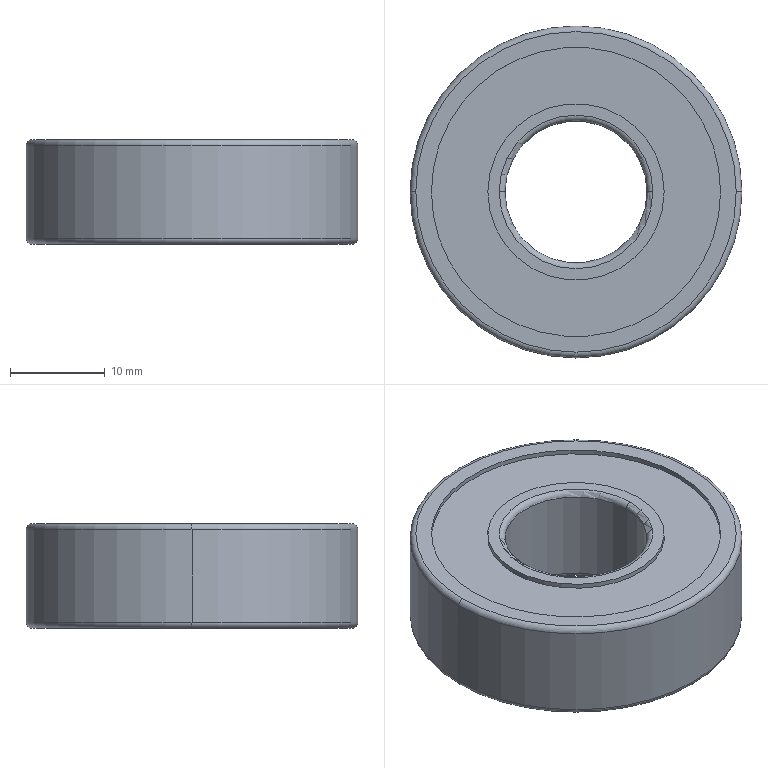Part | STEP file | 6202RS | 3 solids | 26 faces | box 35 x 35 x 11 mm | volume 8156 mm3 | cylinder 12 | torus 8 | plane 6 | commonest cylinder face diameters 18.6 x4 30.5 x4 15 x2 35 x2
STEP:
#1=CARTESIAN_POINT('',(-17.5,0.,10.4));
#2=VERTEX_POINT('',#1);
#3=CARTESIAN_POINT('',(17.5,0.,10.4));
#4=VERTEX_POINT('',#3);
#5=CARTESIAN_POINT('',(0.,0.,10.4));
#6=DIRECTION('',(0.,0.,-1.));
#7=DIRECTION('',(1.,0.,0.));
#8=AXIS2_PLACEMENT_3D('',#5,#6,#7);
#9=CIRCLE('',#8,17.5);
#10=EDGE_CURVE('',#2,#4,#9,.T.);
#11=ORIENTED_EDGE('',*,*,#10,.F.);
#12=CARTESIAN_POINT('',(-16.9,0.,11.));
#13=VERTEX_POINT('',#12);
#14=CARTESIAN_POINT('',(-16.9,0.,10.4));
#15=DIRECTION('',(0.,1.,0.));
#16=DIRECTION('',(-1.,0.,0.));
#17=AXIS2_PLACEMENT_3D('',#14,#15,#16);
#18=CIRCLE('',#17,0.6);
#19=EDGE_CURVE('',#2,#13,#18,.T.);
#20=ORIENTED_EDGE('',*,*,#19,.T.);
#21=CARTESIAN_POINT('',(16.9,0.,11.));
#22=VERTEX_POINT('',#21);
#23=CARTESIAN_POINT('',(0.,0.,11.));
#24=DIRECTION('',(0.,0.,1.));
#25=DIRECTION('',(1.,0.,0.));
#26=AXIS2_PLACEMENT_3D('',#23,#24,#25);
#27=CIRCLE('',#26,16.9);
#28=EDGE_CURVE('',#22,#13,#27,.T.);
#29=ORIENTED_EDGE('',*,*,#28,.F.);
#30=CARTESIAN_POINT('',(16.9,0.,10.4));
#31=DIRECTION('',(0.,-1.,0.));
#32=DIRECTION('',(0.,0.,-1.));
#33=AXIS2_PLACEMENT_3D('',#30,#31,#32);
#34=CIRCLE('',#33,0.6);
#35=EDGE_CURVE('',#4,#22,#34,.T.);
#36=ORIENTED_EDGE('',*,*,#35,.F.);
#37=EDGE_LOOP('',(#11,#20,#29,#36));
#38=FACE_OUTER_BOUND('',#37,.T.);
#39=CARTESIAN_POINT('',(0.,0.,10.4));
#40=DIRECTION('',(0.,0.,1.));
#41=DIRECTION('',(1.,0.,0.));
#42=AXIS2_PLACEMENT_3D('',#39,#40,#41);
#43=TOROIDAL_SURFACE('',#42,16.9,0.6);
#44=ADVANCED_FACE('',(#38),#43,.T.);
#45=CARTESIAN_POINT('',(-16.9,0.,0.));
#46=VERTEX_POINT('',#45);
#47=CARTESIAN_POINT('',(16.9,0.,0.));
#48=VERTEX_POINT('',#47);
#49=CARTESIAN_POINT('',(0.,0.,0.));
#50=DIRECTION('',(0.,0.,-1.));
#51=DIRECTION('',(1.,0.,0.));
#52=AXIS2_PLACEMENT_3D('',#49,#50,#51);
#53=CIRCLE('',#52,16.9);
#54=EDGE_CURVE('',#46,#48,#53,.T.);
#55=ORIENTED_EDGE('',*,*,#54,.F.);
#56=CARTESIAN_POINT('',(-17.5,0.,0.6));
#57=VERTEX_POINT('',#56);
#58=CARTESIAN_POINT('',(-16.9,0.,0.6));
#59=DIRECTION('',(0.,1.,0.));
#60=DIRECTION('',(-1.,0.,0.));
#61=AXIS2_PLACEMENT_3D('',#58,#59,#60);
#62=CIRCLE('',#61,0.6);
#63=EDGE_CURVE('',#46,#57,#62,.T.);
#64=ORIENTED_EDGE('',*,*,#63,.T.);
#65=CARTESIAN_POINT('',(17.5,0.,0.6));
#66=VERTEX_POINT('',#65);
#67=CARTESIAN_POINT('',(0.,0.,0.6));
#68=DIRECTION('',(0.,0.,1.));
#69=DIRECTION('',(1.,0.,0.));
#70=AXIS2_PLACEMENT_3D('',#67,#68,#69);
#71=CIRCLE('',#70,17.5);
#72=EDGE_CURVE('',#66,#57,#71,.T.);
#73=ORIENTED_EDGE('',*,*,#72,.F.);
#74=CARTESIAN_POINT('',(16.9,0.,0.6));
#75=DIRECTION('',(0.,-1.,0.));
#76=DIRECTION('',(0.,0.,-1.));
#77=AXIS2_PLACEMENT_3D('',#74,#75,#76);
#78=CIRCLE('',#77,0.6);
#79=EDGE_CURVE('',#48,#66,#78,.T.);
#80=ORIENTED_EDGE('',*,*,#79,.F.);
#81=EDGE_LOOP('',(#55,#64,#73,#80));
#82=FACE_OUTER_BOUND('',#81,.T.);
#83=CARTESIAN_POINT('',(0.,0.,0.6));
#84=DIRECTION('',(0.,0.,1.));
#85=DIRECTION('',(1.,0.,0.));
#86=AXIS2_PLACEMENT_3D('',#83,#84,#85);
#87=TOROIDAL_SURFACE('',#86,16.9,0.6);
#88=ADVANCED_FACE('',(#82),#87,.T.);
#89=ORIENTED_EDGE('',*,*,#10,.T.);
#90=CARTESIAN_POINT('',(17.5,0.,11.));
#91=DIRECTION('',(0.,0.,-1.));
#92=VECTOR('',#91,1000.);
#93=LINE('',#90,#92);
#94=EDGE_CURVE('',#4,#66,#93,.T.);
#95=ORIENTED_EDGE('',*,*,#94,.T.);
#96=ORIENTED_EDGE('',*,*,#72,.T.);
#97=CARTESIAN_POINT('',(-17.5,0.,11.));
#98=DIRECTION('',(0.,0.,-1.));
#99=VECTOR('',#98,1000.);
#100=LINE('',#97,#99);
#101=EDGE_CURVE('',#2,#57,#100,.T.);
#102=ORIENTED_EDGE('',*,*,#101,.F.);
#103=EDGE_LOOP('',(#89,#95,#96,#102));
#104=FACE_OUTER_BOUND('',#103,.T.);
#105=CARTESIAN_POINT('',(0.,0.,11.));
#106=DIRECTION('',(0.,0.,-1.));
#107=DIRECTION('',(-1.,0.,0.));
#108=AXIS2_PLACEMENT_3D('',#105,#106,#107);
#109=CYLINDRICAL_SURFACE('',#108,17.5);
#110=ADVANCED_FACE('',(#104),#109,.T.);
#111=CARTESIAN_POINT('',(-15.25,0.,11.));
#112=VERTEX_POINT('',#111);
#113=CARTESIAN_POINT('',(15.25,0.,11.));
#114=VERTEX_POINT('',#113);
#115=CARTESIAN_POINT('',(0.,0.,11.));
#116=DIRECTION('',(0.,0.,1.));
#117=DIRECTION('',(1.,0.,0.));
#118=AXIS2_PLACEMENT_3D('',#115,#116,#117);
#119=CIRCLE('',#118,15.25);
#120=EDGE_CURVE('',#112,#114,#119,.T.);
#121=ORIENTED_EDGE('',*,*,#120,.T.);
#122=CARTESIAN_POINT('',(15.25,0.,0.));
#123=VERTEX_POINT('',#122);
#124=CARTESIAN_POINT('',(15.25,0.,11.));
#125=DIRECTION('',(0.,0.,-1.));
#126=VECTOR('',#125,1000.);
#127=LINE('',#124,#126);
#128=EDGE_CURVE('',#114,#123,#127,.T.);
#129=ORIENTED_EDGE('',*,*,#128,.T.);
#130=CARTESIAN_POINT('',(-15.25,0.,0.));
#131=VERTEX_POINT('',#130);
#132=CARTESIAN_POINT('',(0.,0.,0.));
#133=DIRECTION('',(0.,0.,1.));
#134=DIRECTION('',(1.,0.,0.));
#135=AXIS2_PLACEMENT_3D('',#132,#133,#134);
#136=CIRCLE('',#135,15.25);
#137=EDGE_CURVE('',#131,#123,#136,.T.);
#138=ORIENTED_EDGE('',*,*,#137,.F.);
#139=CARTESIAN_POINT('',(-15.25,0.,11.));
#140=DIRECTION('',(0.,0.,-1.));
#141=VECTOR('',#140,1000.);
#142=LINE('',#139,#141);
#143=EDGE_CURVE('',#112,#131,#142,.T.);
#144=ORIENTED_EDGE('',*,*,#143,.F.);
#145=EDGE_LOOP('',(#121,#129,#138,#144));
#146=FACE_OUTER_BOUND('',#145,.T.);
#147=CARTESIAN_POINT('',(0.,0.,11.));
#148=DIRECTION('',(0.,0.,-1.));
#149=DIRECTION('',(-1.,0.,0.));
#150=AXIS2_PLACEMENT_3D('',#147,#148,#149);
#151=CYLINDRICAL_SURFACE('',#150,15.25);
#152=ADVANCED_FACE('',(#146),#151,.F.);
#153=ORIENTED_EDGE('',*,*,#128,.F.);
#154=CARTESIAN_POINT('',(0.,0.,11.));
#155=DIRECTION('',(0.,0.,1.));
#156=DIRECTION('',(1.,0.,0.));
#157=AXIS2_PLACEMENT_3D('',#154,#155,#156);
#158=CIRCLE('',#157,15.25);
#159=EDGE_CURVE('',#114,#112,#158,.T.);
#160=ORIENTED_EDGE('',*,*,#159,.T.);
#161=ORIENTED_EDGE('',*,*,#143,.T.);
#162=CARTESIAN_POINT('',(0.,0.,0.));
#163=DIRECTION('',(0.,0.,1.));
#164=DIRECTION('',(1.,0.,0.));
#165=AXIS2_PLACEMENT_3D('',#162,#163,#164);
#166=CIRCLE('',#165,15.25);
#167=EDGE_CURVE('',#123,#131,#166,.T.);
#168=ORIENTED_EDGE('',*,*,#167,.F.);
#169=EDGE_LOOP('',(#153,#160,#161,#168));
#170=FACE_OUTER_BOUND('',#169,.T.);
#171=CARTESIAN_POINT('',(0.,0.,11.));
#172=DIRECTION('',(0.,0.,-1.));
#173=DIRECTION('',(-1.,0.,0.));
#174=AXIS2_PLACEMENT_3D('',#171,#172,#173);
#175=CYLINDRICAL_SURFACE('',#174,15.25);
#176=ADVANCED_FACE('',(#170),#175,.F.);
#177=ORIENTED_EDGE('',*,*,#94,.F.);
#178=CARTESIAN_POINT('',(0.,0.,10.4));
#179=DIRECTION('',(0.,0.,-1.));
#180=DIRECTION('',(1.,0.,0.));
#181=AXIS2_PLACEMENT_3D('',#178,#179,#180);
#182=CIRCLE('',#181,17.5);
#183=EDGE_CURVE('',#4,#2,#182,.T.);
#184=ORIENTED_EDGE('',*,*,#183,.T.);
#185=ORIENTED_EDGE('',*,*,#101,.T.);
#186=CARTESIAN_POINT('',(0.,0.,0.6));
#187=DIRECTION('',(0.,0.,1.));
#188=DIRECTION('',(1.,0.,0.));
#189=AXIS2_PLACEMENT_3D('',#186,#187,#188);
#190=CIRCLE('',#189,17.5);
#191=EDGE_CURVE('',#57,#66,#190,.T.);
#192=ORIENTED_EDGE('',*,*,#191,.T.);
#193=EDGE_LOOP('',(#177,#184,#185,#192));
#194=FACE_OUTER_BOUND('',#193,.T.);
#195=CARTESIAN_POINT('',(0.,0.,11.));
#196=DIRECTION('',(0.,0.,-1.));
#197=DIRECTION('',(-1.,0.,0.));
#198=AXIS2_PLACEMENT_3D('',#195,#196,#197);
#199=CYLINDRICAL_SURFACE('',#198,17.5);
#200=ADVANCED_FACE('',(#194),#199,.T.);
#201=ORIENTED_EDGE('',*,*,#28,.T.);
#202=CARTESIAN_POINT('',(0.,0.,11.));
#203=DIRECTION('',(0.,0.,1.));
#204=DIRECTION('',(1.,0.,0.));
#205=AXIS2_PLACEMENT_3D('',#202,#203,#204);
#206=CIRCLE('',#205,16.9);
#207=EDGE_CURVE('',#13,#22,#206,.T.);
#208=ORIENTED_EDGE('',*,*,#207,.T.);
#209=EDGE_LOOP('',(#201,#208));
#210=FACE_OUTER_BOUND('',#209,.T.);
#211=ORIENTED_EDGE('',*,*,#120,.F.);
#212=ORIENTED_EDGE('',*,*,#159,.F.);
#213=EDGE_LOOP('',(#211,#212));
#214=FACE_BOUND('',#213,.T.);
#215=CARTESIAN_POINT('',(0.,0.,11.));
#216=DIRECTION('',(0.,0.,1.));
#217=DIRECTION('',(1.,0.,0.));
#218=AXIS2_PLACEMENT_3D('',#215,#216,#217);
#219=PLANE('',#218);
#220=ADVANCED_FACE('',(#210,#214),#219,.T.);
#221=CARTESIAN_POINT('',(0.,0.,0.));
#222=DIRECTION('',(0.,0.,-1.));
#223=DIRECTION('',(1.,0.,0.));
#224=AXIS2_PLACEMENT_3D('',#221,#222,#223);
#225=CIRCLE('',#224,16.9);
#226=EDGE_CURVE('',#48,#46,#225,.T.);
#227=ORIENTED_EDGE('',*,*,#226,.T.);
#228=ORIENTED_EDGE('',*,*,#54,.T.);
#229=EDGE_LOOP('',(#227,#228));
#230=FACE_OUTER_BOUND('',#229,.T.);
#231=ORIENTED_EDGE('',*,*,#137,.T.);
#232=ORIENTED_EDGE('',*,*,#167,.T.);
#233=EDGE_LOOP('',(#231,#232));
#234=FACE_BOUND('',#233,.T.);
#235=CARTESIAN_POINT('',(0.,0.,0.));
#236=DIRECTION('',(0.,0.,1.));
#237=DIRECTION('',(1.,0.,0.));
#238=AXIS2_PLACEMENT_3D('',#235,#236,#237);
#239=PLANE('',#238);
#240=ADVANCED_FACE('',(#230,#234),#239,.F.);
#241=ORIENTED_EDGE('',*,*,#63,.F.);
#242=ORIENTED_EDGE('',*,*,#226,.F.);
#243=ORIENTED_EDGE('',*,*,#79,.T.);
#244=ORIENTED_EDGE('',*,*,#191,.F.);
#245=EDGE_LOOP('',(#241,#242,#243,#244));
#246=FACE_OUTER_BOUND('',#245,.T.);
#247=CARTESIAN_POINT('',(0.,0.,0.6));
#248=DIRECTION('',(0.,0.,1.));
#249=DIRECTION('',(1.,0.,0.));
#250=AXIS2_PLACEMENT_3D('',#247,#248,#249);
#251=TOROIDAL_SURFACE('',#250,16.9,0.6);
#252=ADVANCED_FACE('',(#246),#251,.T.);
#253=ORIENTED_EDGE('',*,*,#19,.F.);
#254=ORIENTED_EDGE('',*,*,#183,.F.);
#255=ORIENTED_EDGE('',*,*,#35,.T.);
#256=ORIENTED_EDGE('',*,*,#207,.F.);
#257=EDGE_LOOP('',(#253,#254,#255,#256));
#258=FACE_OUTER_BOUND('',#257,.T.);
#259=CARTESIAN_POINT('',(0.,0.,10.4));
#260=DIRECTION('',(0.,0.,1.));
#261=DIRECTION('',(1.,0.,0.));
#262=AXIS2_PLACEMENT_3D('',#259,#260,#261);
#263=TOROIDAL_SURFACE('',#262,16.9,0.6);
#264=ADVANCED_FACE('',(#258),#263,.T.);
#265=CLOSED_SHELL('',(#44,#88,#110,#152,#176,#200,#220,#240,#252,#264));
#266=MANIFOLD_SOLID_BREP('',#265);
#267=CARTESIAN_POINT('',(-8.1,0.,11.));
#268=VERTEX_POINT('',#267);
#269=CARTESIAN_POINT('',(8.1,0.,11.));
#270=VERTEX_POINT('',#269);
#271=CARTESIAN_POINT('',(0.,0.,11.));
#272=DIRECTION('',(0.,0.,-1.));
#273=DIRECTION('',(1.,0.,0.));
#274=AXIS2_PLACEMENT_3D('',#271,#272,#273);
#275=CIRCLE('',#274,8.1);
#276=EDGE_CURVE('',#268,#270,#275,.T.);
#277=ORIENTED_EDGE('',*,*,#276,.F.);
#278=CARTESIAN_POINT('',(-7.5,0.,10.4));
#279=VERTEX_POINT('',#278);
#280=CARTESIAN_POINT('',(-8.1,0.,10.4));
#281=DIRECTION('',(0.,1.,0.));
#282=DIRECTION('',(-1.,0.,0.));
#283=AXIS2_PLACEMENT_3D('',#280,#281,#282);
#284=CIRCLE('',#283,0.6);
#285=EDGE_CURVE('',#268,#279,#284,.T.);
#286=ORIENTED_EDGE('',*,*,#285,.T.);
#287=CARTESIAN_POINT('',(7.5,0.,10.4));
#288=VERTEX_POINT('',#287);
#289=CARTESIAN_POINT('',(0.,0.,10.4));
#290=DIRECTION('',(0.,0.,1.));
#291=DIRECTION('',(1.,0.,0.));
#292=AXIS2_PLACEMENT_3D('',#289,#290,#291);
#293=CIRCLE('',#292,7.5);
#294=EDGE_CURVE('',#288,#279,#293,.T.);
#295=ORIENTED_EDGE('',*,*,#294,.F.);
#296=CARTESIAN_POINT('',(8.1,0.,10.4));
#297=DIRECTION('',(0.,-1.,0.));
#298=DIRECTION('',(0.,0.,-1.));
#299=AXIS2_PLACEMENT_3D('',#296,#297,#298);
#300=CIRCLE('',#299,0.6);
#301=EDGE_CURVE('',#270,#288,#300,.T.);
#302=ORIENTED_EDGE('',*,*,#301,.F.);
#303=EDGE_LOOP('',(#277,#286,#295,#302));
#304=FACE_OUTER_BOUND('',#303,.T.);
#305=CARTESIAN_POINT('',(0.,0.,10.4));
#306=DIRECTION('',(0.,0.,1.));
#307=DIRECTION('',(1.,0.,0.));
#308=AXIS2_PLACEMENT_3D('',#305,#306,#307);
#309=TOROIDAL_SURFACE('',#308,8.1,0.6);
#310=ADVANCED_FACE('',(#304),#309,.T.);
#311=CARTESIAN_POINT('',(-7.5,0.,0.6));
#312=VERTEX_POINT('',#311);
#313=CARTESIAN_POINT('',(7.5,0.,0.6));
#314=VERTEX_POINT('',#313);
#315=CARTESIAN_POINT('',(0.,0.,0.6));
#316=DIRECTION('',(0.,0.,-1.));
#317=DIRECTION('',(1.,0.,0.));
#318=AXIS2_PLACEMENT_3D('',#315,#316,#317);
#319=CIRCLE('',#318,7.5);
#320=EDGE_CURVE('',#312,#314,#319,.T.);
#321=ORIENTED_EDGE('',*,*,#320,.F.);
#322=CARTESIAN_POINT('',(-8.1,0.,0.));
#323=VERTEX_POINT('',#322);
#324=CARTESIAN_POINT('',(-8.1,0.,0.6));
#325=DIRECTION('',(0.,1.,0.));
#326=DIRECTION('',(-1.,0.,0.));
#327=AXIS2_PLACEMENT_3D('',#324,#325,#326);
#328=CIRCLE('',#327,0.6);
#329=EDGE_CURVE('',#312,#323,#328,.T.);
#330=ORIENTED_EDGE('',*,*,#329,.T.);
#331=CARTESIAN_POINT('',(8.1,0.,0.));
#332=VERTEX_POINT('',#331);
#333=CARTESIAN_POINT('',(0.,0.,0.));
#334=DIRECTION('',(0.,0.,1.));
#335=DIRECTION('',(1.,0.,0.));
#336=AXIS2_PLACEMENT_3D('',#333,#334,#335);
#337=CIRCLE('',#336,8.1);
#338=EDGE_CURVE('',#332,#323,#337,.T.);
#339=ORIENTED_EDGE('',*,*,#338,.F.);
#340=CARTESIAN_POINT('',(8.1,0.,0.6));
#341=DIRECTION('',(0.,-1.,0.));
#342=DIRECTION('',(0.,0.,-1.));
#343=AXIS2_PLACEMENT_3D('',#340,#341,#342);
#344=CIRCLE('',#343,0.6);
#345=EDGE_CURVE('',#314,#332,#344,.T.);
#346=ORIENTED_EDGE('',*,*,#345,.F.);
#347=EDGE_LOOP('',(#321,#330,#339,#346));
#348=FACE_OUTER_BOUND('',#347,.T.);
#349=CARTESIAN_POINT('',(0.,0.,0.6));
#350=DIRECTION('',(0.,0.,1.));
#351=DIRECTION('',(1.,0.,0.));
#352=AXIS2_PLACEMENT_3D('',#349,#350,#351);
#353=TOROIDAL_SURFACE('',#352,8.1,0.6);
#354=ADVANCED_FACE('',(#348),#353,.T.);
#355=CARTESIAN_POINT('',(9.3,0.,11.));
#356=VERTEX_POINT('',#355);
#357=CARTESIAN_POINT('',(-9.3,0.,11.));
#358=VERTEX_POINT('',#357);
#359=CARTESIAN_POINT('',(0.,0.,11.));
#360=DIRECTION('',(0.,0.,1.));
#361=DIRECTION('',(1.,0.,0.));
#362=AXIS2_PLACEMENT_3D('',#359,#360,#361);
#363=CIRCLE('',#362,9.3);
#364=EDGE_CURVE('',#356,#358,#363,.T.);
#365=ORIENTED_EDGE('',*,*,#364,.F.);
#366=CARTESIAN_POINT('',(9.3,0.,0.));
#367=VERTEX_POINT('',#366);
#368=CARTESIAN_POINT('',(9.3,0.,11.));
#369=DIRECTION('',(0.,0.,-1.));
#370=VECTOR('',#369,1000.);
#371=LINE('',#368,#370);
#372=EDGE_CURVE('',#356,#367,#371,.T.);
#373=ORIENTED_EDGE('',*,*,#372,.T.);
#374=CARTESIAN_POINT('',(-9.3,0.,0.));
#375=VERTEX_POINT('',#374);
#376=CARTESIAN_POINT('',(0.,0.,0.));
#377=DIRECTION('',(0.,0.,1.));
#378=DIRECTION('',(1.,0.,0.));
#379=AXIS2_PLACEMENT_3D('',#376,#377,#378);
#380=CIRCLE('',#379,9.3);
#381=EDGE_CURVE('',#367,#375,#380,.T.);
#382=ORIENTED_EDGE('',*,*,#381,.T.);
#383=CARTESIAN_POINT('',(-9.3,0.,11.));
#384=DIRECTION('',(0.,0.,-1.));
#385=VECTOR('',#384,1000.);
#386=LINE('',#383,#385);
#387=EDGE_CURVE('',#358,#375,#386,.T.);
#388=ORIENTED_EDGE('',*,*,#387,.F.);
#389=EDGE_LOOP('',(#365,#373,#382,#388));
#390=FACE_OUTER_BOUND('',#389,.T.);
#391=CARTESIAN_POINT('',(0.,0.,11.));
#392=DIRECTION('',(0.,0.,-1.));
#393=DIRECTION('',(-1.,0.,0.));
#394=AXIS2_PLACEMENT_3D('',#391,#392,#393);
#395=CYLINDRICAL_SURFACE('',#394,9.3);
#396=ADVANCED_FACE('',(#390),#395,.T.);
#397=CARTESIAN_POINT('',(0.,0.,10.4));
#398=DIRECTION('',(0.,0.,1.));
#399=DIRECTION('',(1.,0.,0.));
#400=AXIS2_PLACEMENT_3D('',#397,#398,#399);
#401=CIRCLE('',#400,7.5);
#402=EDGE_CURVE('',#279,#288,#401,.T.);
#403=ORIENTED_EDGE('',*,*,#402,.T.);
#404=CARTESIAN_POINT('',(7.5,0.,11.));
#405=DIRECTION('',(0.,0.,-1.));
#406=VECTOR('',#405,1000.);
#407=LINE('',#404,#406);
#408=EDGE_CURVE('',#288,#314,#407,.T.);
#409=ORIENTED_EDGE('',*,*,#408,.T.);
#410=CARTESIAN_POINT('',(0.,0.,0.6));
#411=DIRECTION('',(0.,0.,-1.));
#412=DIRECTION('',(1.,0.,0.));
#413=AXIS2_PLACEMENT_3D('',#410,#411,#412);
#414=CIRCLE('',#413,7.5);
#415=EDGE_CURVE('',#314,#312,#414,.T.);
#416=ORIENTED_EDGE('',*,*,#415,.T.);
#417=CARTESIAN_POINT('',(-7.5,0.,11.));
#418=DIRECTION('',(0.,0.,-1.));
#419=VECTOR('',#418,1000.);
#420=LINE('',#417,#419);
#421=EDGE_CURVE('',#279,#312,#420,.T.);
#422=ORIENTED_EDGE('',*,*,#421,.F.);
#423=EDGE_LOOP('',(#403,#409,#416,#422));
#424=FACE_OUTER_BOUND('',#423,.T.);
#425=CARTESIAN_POINT('',(0.,0.,11.));
#426=DIRECTION('',(0.,0.,-1.));
#427=DIRECTION('',(-1.,0.,0.));
#428=AXIS2_PLACEMENT_3D('',#425,#426,#427);
#429=CYLINDRICAL_SURFACE('',#428,7.5);
#430=ADVANCED_FACE('',(#424),#429,.F.);
#431=ORIENTED_EDGE('',*,*,#408,.F.);
#432=ORIENTED_EDGE('',*,*,#294,.T.);
#433=ORIENTED_EDGE('',*,*,#421,.T.);
#434=ORIENTED_EDGE('',*,*,#320,.T.);
#435=EDGE_LOOP('',(#431,#432,#433,#434));
#436=FACE_OUTER_BOUND('',#435,.T.);
#437=CARTESIAN_POINT('',(0.,0.,11.));
#438=DIRECTION('',(0.,0.,-1.));
#439=DIRECTION('',(-1.,0.,0.));
#440=AXIS2_PLACEMENT_3D('',#437,#438,#439);
#441=CYLINDRICAL_SURFACE('',#440,7.5);
#442=ADVANCED_FACE('',(#436),#441,.F.);
#443=ORIENTED_EDGE('',*,*,#372,.F.);
#444=CARTESIAN_POINT('',(0.,0.,11.));
#445=DIRECTION('',(0.,0.,1.));
#446=DIRECTION('',(1.,0.,0.));
#447=AXIS2_PLACEMENT_3D('',#444,#445,#446);
#448=CIRCLE('',#447,9.3);
#449=EDGE_CURVE('',#358,#356,#448,.T.);
#450=ORIENTED_EDGE('',*,*,#449,.F.);
#451=ORIENTED_EDGE('',*,*,#387,.T.);
#452=CARTESIAN_POINT('',(0.,0.,0.));
#453=DIRECTION('',(0.,0.,1.));
#454=DIRECTION('',(1.,0.,0.));
#455=AXIS2_PLACEMENT_3D('',#452,#453,#454);
#456=CIRCLE('',#455,9.3);
#457=EDGE_CURVE('',#375,#367,#456,.T.);
#458=ORIENTED_EDGE('',*,*,#457,.T.);
#459=EDGE_LOOP('',(#443,#450,#451,#458));
#460=FACE_OUTER_BOUND('',#459,.T.);
#461=CARTESIAN_POINT('',(0.,0.,11.));
#462=DIRECTION('',(0.,0.,-1.));
#463=DIRECTION('',(-1.,0.,0.));
#464=AXIS2_PLACEMENT_3D('',#461,#462,#463);
#465=CYLINDRICAL_SURFACE('',#464,9.3);
#466=ADVANCED_FACE('',(#460),#465,.T.);
#467=CARTESIAN_POINT('',(0.,0.,11.));
#468=DIRECTION('',(0.,0.,-1.));
#469=DIRECTION('',(1.,0.,0.));
#470=AXIS2_PLACEMENT_3D('',#467,#468,#469);
#471=CIRCLE('',#470,8.1);
#472=EDGE_CURVE('',#270,#268,#471,.T.);
#473=ORIENTED_EDGE('',*,*,#472,.T.);
#474=ORIENTED_EDGE('',*,*,#276,.T.);
#475=EDGE_LOOP('',(#473,#474));
#476=FACE_BOUND('',#475,.T.);
#477=ORIENTED_EDGE('',*,*,#449,.T.);
#478=ORIENTED_EDGE('',*,*,#364,.T.);
#479=EDGE_LOOP('',(#477,#478));
#480=FACE_OUTER_BOUND('',#479,.T.);
#481=CARTESIAN_POINT('',(0.,0.,11.));
#482=DIRECTION('',(0.,0.,1.));
#483=DIRECTION('',(1.,0.,0.));
#484=AXIS2_PLACEMENT_3D('',#481,#482,#483);
#485=PLANE('',#484);
#486=ADVANCED_FACE('',(#476,#480),#485,.T.);
#487=ORIENTED_EDGE('',*,*,#338,.T.);
#488=CARTESIAN_POINT('',(0.,0.,0.));
#489=DIRECTION('',(0.,0.,1.));
#490=DIRECTION('',(1.,0.,0.));
#491=AXIS2_PLACEMENT_3D('',#488,#489,#490);
#492=CIRCLE('',#491,8.1);
#493=EDGE_CURVE('',#323,#332,#492,.T.);
#494=ORIENTED_EDGE('',*,*,#493,.T.);
#495=EDGE_LOOP('',(#487,#494));
#496=FACE_BOUND('',#495,.T.);
#497=ORIENTED_EDGE('',*,*,#457,.F.);
#498=ORIENTED_EDGE('',*,*,#381,.F.);
#499=EDGE_LOOP('',(#497,#498));
#500=FACE_OUTER_BOUND('',#499,.T.);
#501=CARTESIAN_POINT('',(0.,0.,0.));
#502=DIRECTION('',(0.,0.,1.));
#503=DIRECTION('',(1.,0.,0.));
#504=AXIS2_PLACEMENT_3D('',#501,#502,#503);
#505=PLANE('',#504);
#506=ADVANCED_FACE('',(#496,#500),#505,.F.);
#507=ORIENTED_EDGE('',*,*,#329,.F.);
#508=ORIENTED_EDGE('',*,*,#415,.F.);
#509=ORIENTED_EDGE('',*,*,#345,.T.);
#510=ORIENTED_EDGE('',*,*,#493,.F.);
#511=EDGE_LOOP('',(#507,#508,#509,#510));
#512=FACE_OUTER_BOUND('',#511,.T.);
#513=CARTESIAN_POINT('',(0.,0.,0.6));
#514=DIRECTION('',(0.,0.,1.));
#515=DIRECTION('',(1.,0.,0.));
#516=AXIS2_PLACEMENT_3D('',#513,#514,#515);
#517=TOROIDAL_SURFACE('',#516,8.1,0.6);
#518=ADVANCED_FACE('',(#512),#517,.T.);
#519=ORIENTED_EDGE('',*,*,#285,.F.);
#520=ORIENTED_EDGE('',*,*,#472,.F.);
#521=ORIENTED_EDGE('',*,*,#301,.T.);
#522=ORIENTED_EDGE('',*,*,#402,.F.);
#523=EDGE_LOOP('',(#519,#520,#521,#522));
#524=FACE_OUTER_BOUND('',#523,.T.);
#525=CARTESIAN_POINT('',(0.,0.,10.4));
#526=DIRECTION('',(0.,0.,1.));
#527=DIRECTION('',(1.,0.,0.));
#528=AXIS2_PLACEMENT_3D('',#525,#526,#527);
#529=TOROIDAL_SURFACE('',#528,8.1,0.6);
#530=ADVANCED_FACE('',(#524),#529,.T.);
#531=CLOSED_SHELL('',(#310,#354,#396,#430,#442,#466,#486,#506,#518,#530));
#532=MANIFOLD_SOLID_BREP('',#531);
#533=CARTESIAN_POINT('',(15.25,0.,10.5));
#534=VERTEX_POINT('',#533);
#535=CARTESIAN_POINT('',(-15.25,0.,10.5));
#536=VERTEX_POINT('',#535);
#537=CARTESIAN_POINT('',(0.,0.,10.5));
#538=DIRECTION('',(0.,0.,1.));
#539=DIRECTION('',(1.,0.,0.));
#540=AXIS2_PLACEMENT_3D('',#537,#538,#539);
#541=CIRCLE('',#540,15.25);
#542=EDGE_CURVE('',#534,#536,#541,.T.);
#543=ORIENTED_EDGE('',*,*,#542,.F.);
#544=CARTESIAN_POINT('',(15.25,0.,0.5));
#545=VERTEX_POINT('',#544);
#546=CARTESIAN_POINT('',(15.25,0.,10.5));
#547=DIRECTION('',(0.,0.,-1.));
#548=VECTOR('',#547,1000.);
#549=LINE('',#546,#548);
#550=EDGE_CURVE('',#534,#545,#549,.T.);
#551=ORIENTED_EDGE('',*,*,#550,.T.);
#552=CARTESIAN_POINT('',(-15.25,0.,0.5));
#553=VERTEX_POINT('',#552);
#554=CARTESIAN_POINT('',(0.,0.,0.5));
#555=DIRECTION('',(0.,0.,1.));
#556=DIRECTION('',(1.,0.,0.));
#557=AXIS2_PLACEMENT_3D('',#554,#555,#556);
#558=CIRCLE('',#557,15.25);
#559=EDGE_CURVE('',#545,#553,#558,.T.);
#560=ORIENTED_EDGE('',*,*,#559,.T.);
#561=CARTESIAN_POINT('',(-15.25,0.,10.5));
#562=DIRECTION('',(0.,0.,-1.));
#563=VECTOR('',#562,1000.);
#564=LINE('',#561,#563);
#565=EDGE_CURVE('',#536,#553,#564,.T.);
#566=ORIENTED_EDGE('',*,*,#565,.F.);
#567=EDGE_LOOP('',(#543,#551,#560,#566));
#568=FACE_OUTER_BOUND('',#567,.T.);
#569=CARTESIAN_POINT('',(0.,0.,10.5));
#570=DIRECTION('',(0.,0.,-1.));
#571=DIRECTION('',(-1.,0.,0.));
#572=AXIS2_PLACEMENT_3D('',#569,#570,#571);
#573=CYLINDRICAL_SURFACE('',#572,15.25);
#574=ADVANCED_FACE('',(#568),#573,.T.);
#575=CARTESIAN_POINT('',(-9.3,0.,10.5));
#576=VERTEX_POINT('',#575);
#577=CARTESIAN_POINT('',(9.3,0.,10.5));
#578=VERTEX_POINT('',#577);
#579=CARTESIAN_POINT('',(0.,0.,10.5));
#580=DIRECTION('',(0.,0.,1.));
#581=DIRECTION('',(1.,0.,0.));
#582=AXIS2_PLACEMENT_3D('',#579,#580,#581);
#583=CIRCLE('',#582,9.3);
#584=EDGE_CURVE('',#576,#578,#583,.T.);
#585=ORIENTED_EDGE('',*,*,#584,.T.);
#586=CARTESIAN_POINT('',(9.3,0.,0.5));
#587=VERTEX_POINT('',#586);
#588=CARTESIAN_POINT('',(9.3,0.,10.5));
#589=DIRECTION('',(0.,0.,-1.));
#590=VECTOR('',#589,1000.);
#591=LINE('',#588,#590);
#592=EDGE_CURVE('',#578,#587,#591,.T.);
#593=ORIENTED_EDGE('',*,*,#592,.T.);
#594=CARTESIAN_POINT('',(-9.3,0.,0.5));
#595=VERTEX_POINT('',#594);
#596=CARTESIAN_POINT('',(0.,0.,0.5));
#597=DIRECTION('',(0.,0.,1.));
#598=DIRECTION('',(1.,0.,0.));
#599=AXIS2_PLACEMENT_3D('',#596,#597,#598);
#600=CIRCLE('',#599,9.3);
#601=EDGE_CURVE('',#595,#587,#600,.T.);
#602=ORIENTED_EDGE('',*,*,#601,.F.);
#603=CARTESIAN_POINT('',(-9.3,0.,10.5));
#604=DIRECTION('',(0.,0.,-1.));
#605=VECTOR('',#604,1000.);
#606=LINE('',#603,#605);
#607=EDGE_CURVE('',#576,#595,#606,.T.);
#608=ORIENTED_EDGE('',*,*,#607,.F.);
#609=EDGE_LOOP('',(#585,#593,#602,#608));
#610=FACE_OUTER_BOUND('',#609,.T.);
#611=CARTESIAN_POINT('',(0.,0.,10.5));
#612=DIRECTION('',(0.,0.,-1.));
#613=DIRECTION('',(-1.,0.,0.));
#614=AXIS2_PLACEMENT_3D('',#611,#612,#613);
#615=CYLINDRICAL_SURFACE('',#614,9.3);
#616=ADVANCED_FACE('',(#610),#615,.F.);
#617=ORIENTED_EDGE('',*,*,#592,.F.);
#618=CARTESIAN_POINT('',(0.,0.,10.5));
#619=DIRECTION('',(0.,0.,1.));
#620=DIRECTION('',(1.,0.,0.));
#621=AXIS2_PLACEMENT_3D('',#618,#619,#620);
#622=CIRCLE('',#621,9.3);
#623=EDGE_CURVE('',#578,#576,#622,.T.);
#624=ORIENTED_EDGE('',*,*,#623,.T.);
#625=ORIENTED_EDGE('',*,*,#607,.T.);
#626=CARTESIAN_POINT('',(0.,0.,0.5));
#627=DIRECTION('',(0.,0.,1.));
#628=DIRECTION('',(1.,0.,0.));
#629=AXIS2_PLACEMENT_3D('',#626,#627,#628);
#630=CIRCLE('',#629,9.3);
#631=EDGE_CURVE('',#587,#595,#630,.T.);
#632=ORIENTED_EDGE('',*,*,#631,.F.);
#633=EDGE_LOOP('',(#617,#624,#625,#632));
#634=FACE_OUTER_BOUND('',#633,.T.);
#635=CARTESIAN_POINT('',(0.,0.,10.5));
#636=DIRECTION('',(0.,0.,-1.));
#637=DIRECTION('',(-1.,0.,0.));
#638=AXIS2_PLACEMENT_3D('',#635,#636,#637);
#639=CYLINDRICAL_SURFACE('',#638,9.3);
#640=ADVANCED_FACE('',(#634),#639,.F.);
#641=ORIENTED_EDGE('',*,*,#550,.F.);
#642=CARTESIAN_POINT('',(0.,0.,10.5));
#643=DIRECTION('',(0.,0.,1.));
#644=DIRECTION('',(1.,0.,0.));
#645=AXIS2_PLACEMENT_3D('',#642,#643,#644);
#646=CIRCLE('',#645,15.25);
#647=EDGE_CURVE('',#536,#534,#646,.T.);
#648=ORIENTED_EDGE('',*,*,#647,.F.);
#649=ORIENTED_EDGE('',*,*,#565,.T.);
#650=CARTESIAN_POINT('',(0.,0.,0.5));
#651=DIRECTION('',(0.,0.,1.));
#652=DIRECTION('',(1.,0.,0.));
#653=AXIS2_PLACEMENT_3D('',#650,#651,#652);
#654=CIRCLE('',#653,15.25);
#655=EDGE_CURVE('',#553,#545,#654,.T.);
#656=ORIENTED_EDGE('',*,*,#655,.T.);
#657=EDGE_LOOP('',(#641,#648,#649,#656));
#658=FACE_OUTER_BOUND('',#657,.T.);
#659=CARTESIAN_POINT('',(0.,0.,10.5));
#660=DIRECTION('',(0.,0.,-1.));
#661=DIRECTION('',(-1.,0.,0.));
#662=AXIS2_PLACEMENT_3D('',#659,#660,#661);
#663=CYLINDRICAL_SURFACE('',#662,15.25);
#664=ADVANCED_FACE('',(#658),#663,.T.);
#665=ORIENTED_EDGE('',*,*,#584,.F.);
#666=ORIENTED_EDGE('',*,*,#623,.F.);
#667=EDGE_LOOP('',(#665,#666));
#668=FACE_BOUND('',#667,.T.);
#669=ORIENTED_EDGE('',*,*,#647,.T.);
#670=ORIENTED_EDGE('',*,*,#542,.T.);
#671=EDGE_LOOP('',(#669,#670));
#672=FACE_OUTER_BOUND('',#671,.T.);
#673=CARTESIAN_POINT('',(0.,0.,10.5));
#674=DIRECTION('',(0.,0.,1.));
#675=DIRECTION('',(1.,0.,0.));
#676=AXIS2_PLACEMENT_3D('',#673,#674,#675);
#677=PLANE('',#676);
#678=ADVANCED_FACE('',(#668,#672),#677,.T.);
#679=ORIENTED_EDGE('',*,*,#601,.T.);
#680=ORIENTED_EDGE('',*,*,#631,.T.);
#681=EDGE_LOOP('',(#679,#680));
#682=FACE_BOUND('',#681,.T.);
#683=ORIENTED_EDGE('',*,*,#655,.F.);
#684=ORIENTED_EDGE('',*,*,#559,.F.);
#685=EDGE_LOOP('',(#683,#684));
#686=FACE_OUTER_BOUND('',#685,.T.);
#687=CARTESIAN_POINT('',(0.,0.,0.5));
#688=DIRECTION('',(0.,0.,1.));
#689=DIRECTION('',(1.,0.,0.));
#690=AXIS2_PLACEMENT_3D('',#687,#688,#689);
#691=PLANE('',#690);
#692=ADVANCED_FACE('',(#682,#686),#691,.F.);
#693=CLOSED_SHELL('',(#574,#616,#640,#664,#678,#692));
#694=MANIFOLD_SOLID_BREP('',#693);
#695=CARTESIAN_POINT('',(0.,0.,0.));
#696=DIRECTION('',(0.,0.,1.));
#697=DIRECTION('',(1.,0.,0.));
#698=AXIS2_PLACEMENT_3D('',#695,#696,#697);
#699=(LENGTH_UNIT()NAMED_UNIT(*)SI_UNIT(.MILLI.,.METRE.));
#700=UNCERTAINTY_MEASURE_WITH_UNIT(LENGTH_MEASURE(0.00001),#699,'','');
#701=(NAMED_UNIT(*)PLANE_ANGLE_UNIT()SI_UNIT($,.RADIAN.));
#702=(NAMED_UNIT(*)SI_UNIT($,.STERADIAN.)SOLID_ANGLE_UNIT());
#703=(GEOMETRIC_REPRESENTATION_CONTEXT(3)GLOBAL_UNCERTAINTY_ASSIGNED_CONTEXT((#700))GLOBAL_UNIT_ASSIGNED_CONTEXT((#699,#701,#702))REPRESENTATION_CONTEXT('',''));
#704=ADVANCED_BREP_SHAPE_REPRESENTATION('',(#266,#532,#694,#698),#703);